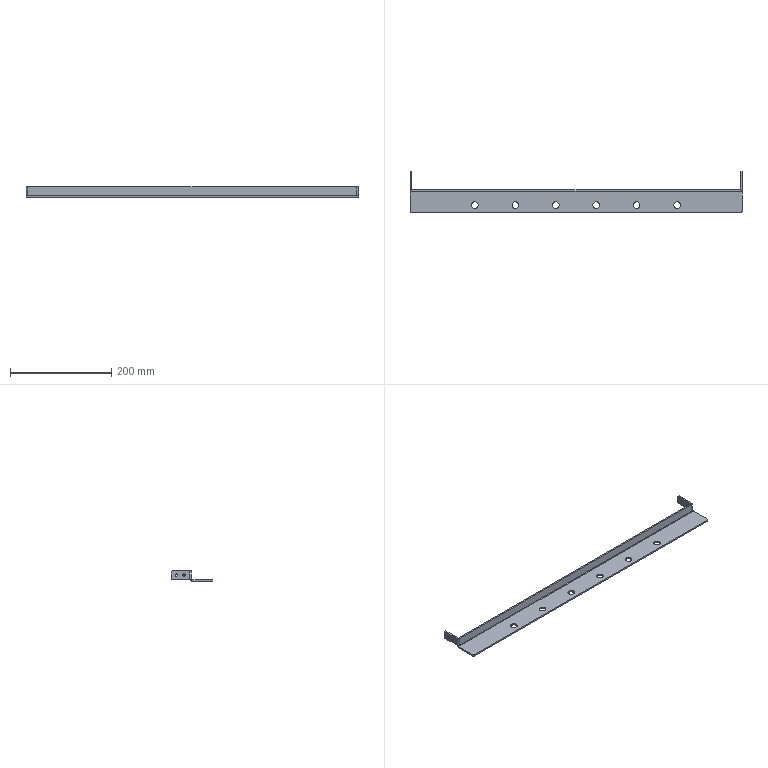Part | STEP file | LM-05-1212_default | 1 solid | 58 faces | box 656 x 82 x 20 mm | volume 121048 mm3 | cylinder 32 | plane 26 | commonest cylinder face diameters 13 x12 4.5 x8 4 x6 1.473 x3 7.473 x3